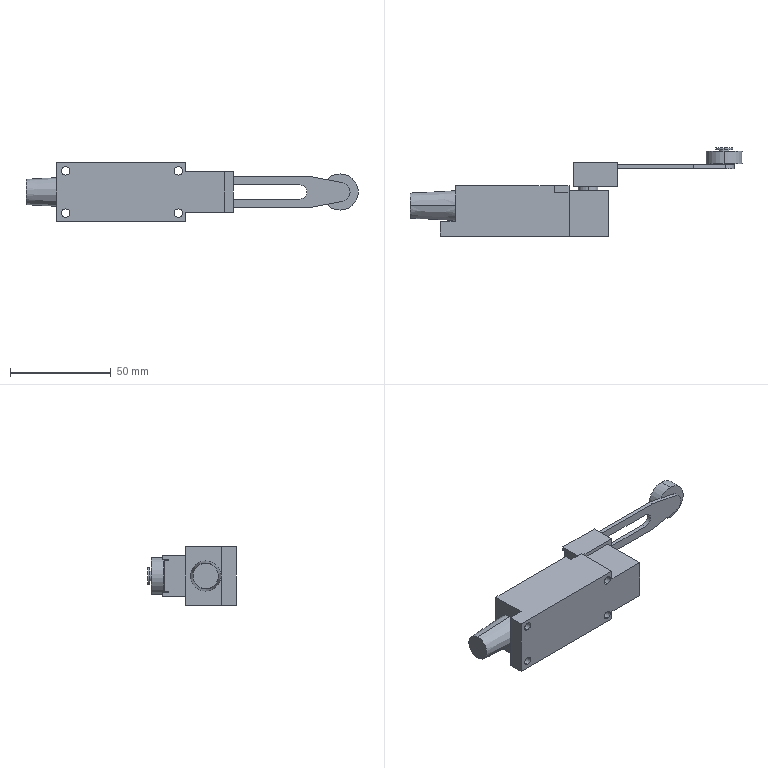Part | SolidWorks | features ICE 15, Extrusion 1, Fillet 1, MirrorPattern 1 | 1 solid | 71 faces | box 165 x 44 x 29 mm | volume 60919 mm3 | plane 47 | cylinder 22 | cone 2 | commonest cylinder face diameters 4.2 x8 5 x4 10 x4 7 x2 8.5 x2 18 x2